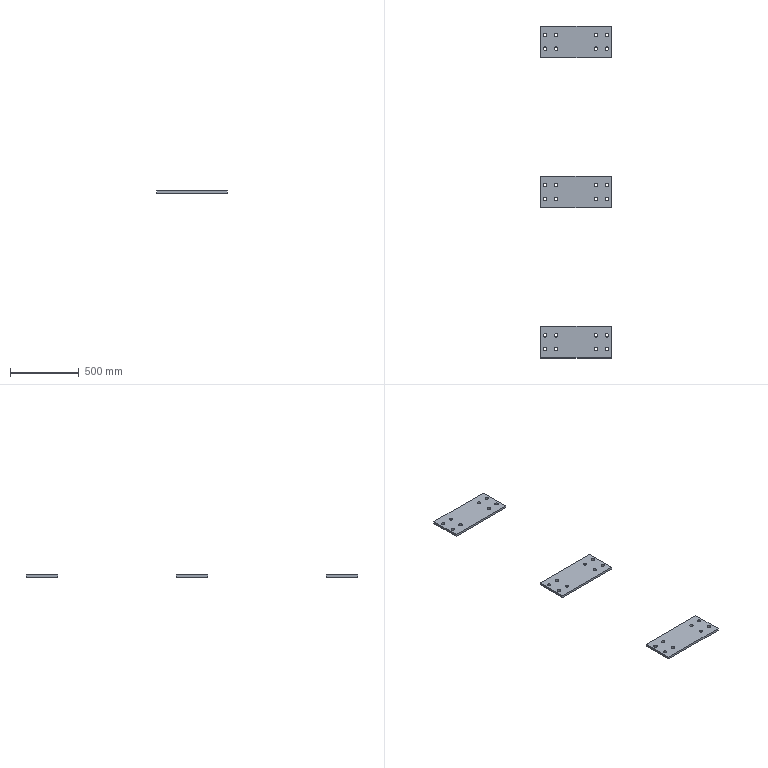Part | STEP file | Plate 510x230x16 | 3 solids | 66 faces | box 510 x 2414 x 16 mm | volume 5441904 mm3 | cylinder 48 | plane 18 | commonest cylinder face diameters 25 x48